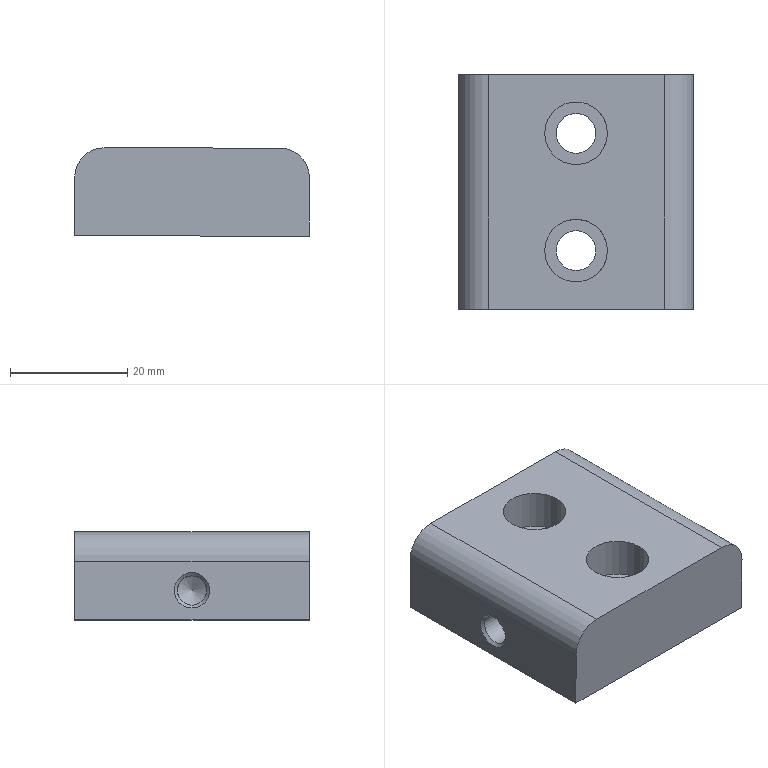Part | STEP file | 冲床-300配套压波_id690_x_t | 1 solid | 18 faces | box 40.015 x 40 x 15.054 mm | volume 21445 mm3 | plane 8 | cylinder 7 | cone 2 | spline 1 | commonest cylinder face diameters 6.8 x2 10 x2 10.7 x2 5 x1
STEP:
#1=CARTESIAN_POINT('',(2190.116,10.,-397.711));
#2=VERTEX_POINT('',#1);
#3=CARTESIAN_POINT('',(2193.516,10.,-397.716));
#4=DIRECTION('',(0.001532,0.,1.));
#5=DIRECTION('',(-1.,0.,0.001532));
#6=AXIS2_PLACEMENT_3D('',#3,#4,#5);
#7=CIRCLE('',#6,3.4);
#8=EDGE_CURVE('',#2,#2,#7,.T.);
#9=ORIENTED_EDGE('',*,*,#8,.F.);
#10=EDGE_LOOP('',(#9));
#11=FACE_BOUND('',#10,.T.);
#12=CARTESIAN_POINT('',(2188.166,10.,-397.708));
#13=VERTEX_POINT('',#12);
#14=CARTESIAN_POINT('',(2193.516,10.,-397.716));
#15=DIRECTION('',(0.001532,0.,1.));
#16=DIRECTION('',(-1.,0.,0.001532));
#17=AXIS2_PLACEMENT_3D('',#14,#15,#16);
#18=CIRCLE('',#17,5.35);
#19=EDGE_CURVE('',#13,#13,#18,.T.);
#20=ORIENTED_EDGE('',*,*,#19,.T.);
#21=EDGE_LOOP('',(#20));
#22=FACE_BOUND('',#21,.T.);
#23=CARTESIAN_POINT('',(2193.516,10.,-397.716));
#24=DIRECTION('',(-0.001532,0.,-1.));
#25=DIRECTION('',(-1.,0.,0.001532));
#26=AXIS2_PLACEMENT_3D('',#23,#24,#25);
#27=PLANE('',#26);
#28=ADVANCED_FACE('',(#11,#22),#27,.F.);
#29=CARTESIAN_POINT('',(2190.103,10.,-405.911));
#30=VERTEX_POINT('',#29);
#31=CARTESIAN_POINT('',(2193.503,10.,-405.916));
#32=DIRECTION('',(0.001532,0.,1.));
#33=DIRECTION('',(-1.,0.,0.001532));
#34=AXIS2_PLACEMENT_3D('',#31,#32,#33);
#35=CIRCLE('',#34,3.4);
#36=EDGE_CURVE('',#30,#30,#35,.T.);
#37=ORIENTED_EDGE('',*,*,#36,.F.);
#38=EDGE_LOOP('',(#37));
#39=FACE_BOUND('',#38,.T.);
#40=ORIENTED_EDGE('',*,*,#8,.T.);
#41=EDGE_LOOP('',(#40));
#42=FACE_BOUND('',#41,.T.);
#43=CARTESIAN_POINT('',(2193.449,10.,-440.916));
#44=DIRECTION('',(-0.001532,0.,-1.));
#45=DIRECTION('',(-1.,0.,0.001532));
#46=AXIS2_PLACEMENT_3D('',#43,#44,#45);
#47=CYLINDRICAL_SURFACE('',#46,3.4);
#48=ADVANCED_FACE('',(#39,#42),#47,.F.);
#49=ORIENTED_EDGE('',*,*,#19,.F.);
#50=EDGE_LOOP('',(#49));
#51=FACE_BOUND('',#50,.T.);
#52=CARTESIAN_POINT('',(2188.176,10.,-390.908));
#53=VERTEX_POINT('',#52);
#54=CARTESIAN_POINT('',(2193.526,10.,-390.916));
#55=DIRECTION('',(-0.001532,0.,-1.));
#56=DIRECTION('',(-1.,0.,0.001532));
#57=AXIS2_PLACEMENT_3D('',#54,#55,#56);
#58=CIRCLE('',#57,5.35);
#59=EDGE_CURVE('',#53,#53,#58,.T.);
#60=ORIENTED_EDGE('',*,*,#59,.F.);
#61=EDGE_LOOP('',(#60));
#62=FACE_BOUND('',#61,.T.);
#63=CARTESIAN_POINT('',(2193.526,10.,-390.916));
#64=DIRECTION('',(-0.001532,0.,-1.));
#65=DIRECTION('',(-1.,0.,0.001532));
#66=AXIS2_PLACEMENT_3D('',#63,#64,#65);
#67=CYLINDRICAL_SURFACE('',#66,5.35);
#68=ADVANCED_FACE('',(#51,#62),#67,.F.);
#69=CARTESIAN_POINT('',(2190.116,-10.,-397.711));
#70=VERTEX_POINT('',#69);
#71=CARTESIAN_POINT('',(2193.516,-10.,-397.716));
#72=DIRECTION('',(0.001532,0.,1.));
#73=DIRECTION('',(-1.,0.,0.001532));
#74=AXIS2_PLACEMENT_3D('',#71,#72,#73);
#75=CIRCLE('',#74,3.4);
#76=EDGE_CURVE('',#70,#70,#75,.T.);
#77=ORIENTED_EDGE('',*,*,#76,.F.);
#78=EDGE_LOOP('',(#77));
#79=FACE_BOUND('',#78,.T.);
#80=CARTESIAN_POINT('',(2188.166,-10.,-397.708));
#81=VERTEX_POINT('',#80);
#82=CARTESIAN_POINT('',(2193.516,-10.,-397.716));
#83=DIRECTION('',(0.001532,0.,1.));
#84=DIRECTION('',(-1.,0.,0.001532));
#85=AXIS2_PLACEMENT_3D('',#82,#83,#84);
#86=CIRCLE('',#85,5.35);
#87=EDGE_CURVE('',#81,#81,#86,.T.);
#88=ORIENTED_EDGE('',*,*,#87,.T.);
#89=EDGE_LOOP('',(#88));
#90=FACE_BOUND('',#89,.T.);
#91=CARTESIAN_POINT('',(2193.516,10.,-397.716));
#92=DIRECTION('',(-0.001532,0.,-1.));
#93=DIRECTION('',(-1.,0.,0.001532));
#94=AXIS2_PLACEMENT_3D('',#91,#92,#93);
#95=PLANE('',#94);
#96=ADVANCED_FACE('',(#79,#90),#95,.F.);
#97=CARTESIAN_POINT('',(2208.526,20.,-390.939));
#98=VERTEX_POINT('',#97);
#99=CARTESIAN_POINT('',(2178.526,20.,-390.893));
#100=VERTEX_POINT('',#99);
#101=CARTESIAN_POINT('',(2203.526,20.,-390.931));
#102=DIRECTION('',(-1.,0.,0.001532));
#103=VECTOR('',#102,1.);
#104=LINE('',#101,#103);
#105=EDGE_CURVE('',#98,#100,#104,.T.);
#106=ORIENTED_EDGE('',*,*,#105,.F.);
#107=CARTESIAN_POINT('',(2213.518,20.,-395.947));
#108=VERTEX_POINT('',#107);
#109=CARTESIAN_POINT('',(2208.518,20.,-395.939));
#110=DIRECTION('',(0.,1.,0.));
#111=DIRECTION('',(0.3358,0.,-0.9419));
#112=AXIS2_PLACEMENT_3D('',#109,#110,#111);
#113=CIRCLE('',#112,5.);
#114=EDGE_CURVE('',#98,#108,#113,.T.);
#115=ORIENTED_EDGE('',*,*,#114,.T.);
#116=CARTESIAN_POINT('',(2213.503,20.,-405.947));
#117=VERTEX_POINT('',#116);
#118=CARTESIAN_POINT('',(2213.503,20.,-405.947));
#119=DIRECTION('',(-0.001532,0.,-1.));
#120=VECTOR('',#119,1.);
#121=LINE('',#118,#120);
#122=EDGE_CURVE('',#108,#117,#121,.T.);
#123=ORIENTED_EDGE('',*,*,#122,.T.);
#124=CARTESIAN_POINT('',(2173.503,20.,-405.885));
#125=VERTEX_POINT('',#124);
#126=CARTESIAN_POINT('',(2203.503,20.,-405.931));
#127=DIRECTION('',(-1.,0.,0.001532));
#128=VECTOR('',#127,1.);
#129=LINE('',#126,#128);
#130=EDGE_CURVE('',#117,#125,#129,.T.);
#131=ORIENTED_EDGE('',*,*,#130,.T.);
#132=CARTESIAN_POINT('',(2173.518,20.,-395.885));
#133=VERTEX_POINT('',#132);
#134=CARTESIAN_POINT('',(2173.503,20.,-405.885));
#135=DIRECTION('',(0.001532,0.,1.));
#136=VECTOR('',#135,1.);
#137=LINE('',#134,#136);
#138=EDGE_CURVE('',#125,#133,#137,.T.);
#139=ORIENTED_EDGE('',*,*,#138,.T.);
#140=CARTESIAN_POINT('',(2178.518,20.,-395.893));
#141=DIRECTION('',(0.,1.,0.));
#142=DIRECTION('',(0.3358,0.,-0.9419));
#143=AXIS2_PLACEMENT_3D('',#140,#141,#142);
#144=CIRCLE('',#143,5.);
#145=EDGE_CURVE('',#133,#100,#144,.T.);
#146=ORIENTED_EDGE('',*,*,#145,.T.);
#147=EDGE_LOOP('',(#106,#115,#123,#131,#139,#146));
#148=FACE_OUTER_BOUND('',#147,.T.);
#149=CARTESIAN_POINT('',(2203.503,20.,-405.931));
#150=DIRECTION('',(0.,-1.,0.));
#151=DIRECTION('',(1.,0.,-0.001532));
#152=AXIS2_PLACEMENT_3D('',#149,#150,#151);
#153=PLANE('',#152);
#154=ADVANCED_FACE('',(#148),#153,.F.);
#155=CARTESIAN_POINT('',(2173.518,-20.,-395.885));
#156=VERTEX_POINT('',#155);
#157=CARTESIAN_POINT('',(2173.518,15.,-395.885));
#158=DIRECTION('',(0.,1.,0.));
#159=VECTOR('',#158,1.);
#160=LINE('',#157,#159);
#161=EDGE_CURVE('',#156,#133,#160,.T.);
#162=ORIENTED_EDGE('',*,*,#161,.T.);
#163=ORIENTED_EDGE('',*,*,#138,.F.);
#164=CARTESIAN_POINT('',(2173.503,-20.,-405.885));
#165=VERTEX_POINT('',#164);
#166=CARTESIAN_POINT('',(2173.503,15.,-405.885));
#167=DIRECTION('',(0.,-1.,0.));
#168=VECTOR('',#167,1.);
#169=LINE('',#166,#168);
#170=EDGE_CURVE('',#125,#165,#169,.T.);
#171=ORIENTED_EDGE('',*,*,#170,.T.);
#172=CARTESIAN_POINT('',(2173.503,-20.,-405.885));
#173=DIRECTION('',(0.001532,0.,1.));
#174=VECTOR('',#173,1.);
#175=LINE('',#172,#174);
#176=EDGE_CURVE('',#165,#156,#175,.T.);
#177=ORIENTED_EDGE('',*,*,#176,.T.);
#178=EDGE_LOOP('',(#162,#163,#171,#177));
#179=FACE_BOUND('',#178,.T.);
#180=CARTESIAN_POINT('',(2173.517,-1.657,-398.382));
#181=VERTEX_POINT('',#180);
#182=CARTESIAN_POINT('',(2173.517,1.658,-398.383));
#183=VERTEX_POINT('',#182);
#184=CARTESIAN_POINT('',(2173.511,0.,-400.885));
#185=DIRECTION('',(1.,0.,-0.001532));
#186=DIRECTION('',(-0.001532,0.,-1.));
#187=AXIS2_PLACEMENT_3D('',#184,#185,#186);
#188=CIRCLE('',#187,3.004);
#189=EDGE_CURVE('',#181,#183,#188,.T.);
#190=ORIENTED_EDGE('',*,*,#189,.T.);
#191=CARTESIAN_POINT('',(2173.515,1.66,-398.381));
#192=CARTESIAN_POINT('',(2173.515,1.427,-398.195));
#193=CARTESIAN_POINT('',(2173.515,1.158,-398.046));
#194=CARTESIAN_POINT('',(2173.515,0.8765,-397.947));
#195=CARTESIAN_POINT('',(2173.515,0.7375,-397.898));
#196=CARTESIAN_POINT('',(2173.515,0.594,-397.861));
#197=CARTESIAN_POINT('',(2173.515,0.4488,-397.836));
#198=CARTESIAN_POINT('',(2173.516,0.1563,-397.786));
#199=CARTESIAN_POINT('',(2173.516,-0.1488,-397.786));
#200=CARTESIAN_POINT('',(2173.515,-0.4414,-397.835));
#201=CARTESIAN_POINT('',(2173.515,-0.7342,-397.885));
#202=CARTESIAN_POINT('',(2173.515,-1.022,-397.985));
#203=CARTESIAN_POINT('',(2173.515,-1.282,-398.129));
#204=CARTESIAN_POINT('',(2173.515,-1.414,-398.202));
#205=CARTESIAN_POINT('',(2173.515,-1.541,-398.286));
#206=CARTESIAN_POINT('',(2173.515,-1.659,-398.381));
#207=B_SPLINE_CURVE_WITH_KNOTS('',3,(#191,#192,#193,#194,#195,#196,#197,#198,#199,#200,#201,#202,#203,#204,#205,#206),.UNSPECIFIED.,.F.,.F.,(4,3,3,3,3,4),(0.,0.2513,0.3739,0.6237,0.8736,1.),.UNSPECIFIED.);
#208=EDGE_CURVE('',#183,#181,#207,.T.);
#209=ORIENTED_EDGE('',*,*,#208,.T.);
#210=EDGE_LOOP('',(#190,#209));
#211=FACE_BOUND('',#210,.T.);
#212=CARTESIAN_POINT('',(2173.503,15.,-405.885));
#213=DIRECTION('',(1.,0.,-0.001532));
#214=DIRECTION('',(0.,-1.,0.));
#215=AXIS2_PLACEMENT_3D('',#212,#213,#214);
#216=PLANE('',#215);
#217=ADVANCED_FACE('',(#179,#211),#216,.F.);
#218=CARTESIAN_POINT('',(2213.518,-20.,-395.947));
#219=VERTEX_POINT('',#218);
#220=CARTESIAN_POINT('',(2213.503,-20.,-405.947));
#221=VERTEX_POINT('',#220);
#222=CARTESIAN_POINT('',(2213.503,-20.,-405.947));
#223=DIRECTION('',(-0.001532,0.,-1.));
#224=VECTOR('',#223,1.);
#225=LINE('',#222,#224);
#226=EDGE_CURVE('',#219,#221,#225,.T.);
#227=ORIENTED_EDGE('',*,*,#226,.F.);
#228=CARTESIAN_POINT('',(2208.526,-20.,-390.939));
#229=VERTEX_POINT('',#228);
#230=CARTESIAN_POINT('',(2208.518,-20.,-395.939));
#231=DIRECTION('',(0.,-1.,0.));
#232=DIRECTION('',(0.3358,0.,-0.9419));
#233=AXIS2_PLACEMENT_3D('',#230,#231,#232);
#234=CIRCLE('',#233,5.);
#235=EDGE_CURVE('',#219,#229,#234,.T.);
#236=ORIENTED_EDGE('',*,*,#235,.T.);
#237=CARTESIAN_POINT('',(2178.526,-20.,-390.893));
#238=VERTEX_POINT('',#237);
#239=CARTESIAN_POINT('',(2203.526,-20.,-390.931));
#240=DIRECTION('',(-1.,0.,0.001532));
#241=VECTOR('',#240,1.);
#242=LINE('',#239,#241);
#243=EDGE_CURVE('',#229,#238,#242,.T.);
#244=ORIENTED_EDGE('',*,*,#243,.T.);
#245=CARTESIAN_POINT('',(2178.518,-20.,-395.893));
#246=DIRECTION('',(0.,-1.,0.));
#247=DIRECTION('',(0.3358,0.,-0.9419));
#248=AXIS2_PLACEMENT_3D('',#245,#246,#247);
#249=CIRCLE('',#248,5.);
#250=EDGE_CURVE('',#238,#156,#249,.T.);
#251=ORIENTED_EDGE('',*,*,#250,.T.);
#252=ORIENTED_EDGE('',*,*,#176,.F.);
#253=CARTESIAN_POINT('',(2203.503,-20.,-405.931));
#254=DIRECTION('',(-1.,0.,0.001532));
#255=VECTOR('',#254,1.);
#256=LINE('',#253,#255);
#257=EDGE_CURVE('',#221,#165,#256,.T.);
#258=ORIENTED_EDGE('',*,*,#257,.F.);
#259=EDGE_LOOP('',(#227,#236,#244,#251,#252,#258));
#260=FACE_OUTER_BOUND('',#259,.T.);
#261=CARTESIAN_POINT('',(2203.503,-20.,-405.931));
#262=DIRECTION('',(0.,-1.,0.));
#263=DIRECTION('',(1.,0.,-0.001532));
#264=AXIS2_PLACEMENT_3D('',#261,#262,#263);
#265=PLANE('',#264);
#266=ADVANCED_FACE('',(#260),#265,.T.);
#267=ORIENTED_EDGE('',*,*,#122,.F.);
#268=CARTESIAN_POINT('',(2213.518,15.,-395.947));
#269=DIRECTION('',(0.,-1.,0.));
#270=VECTOR('',#269,1.);
#271=LINE('',#268,#270);
#272=EDGE_CURVE('',#108,#219,#271,.T.);
#273=ORIENTED_EDGE('',*,*,#272,.T.);
#274=ORIENTED_EDGE('',*,*,#226,.T.);
#275=CARTESIAN_POINT('',(2213.503,15.,-405.947));
#276=DIRECTION('',(0.,1.,0.));
#277=VECTOR('',#276,1.);
#278=LINE('',#275,#277);
#279=EDGE_CURVE('',#221,#117,#278,.T.);
#280=ORIENTED_EDGE('',*,*,#279,.T.);
#281=EDGE_LOOP('',(#267,#273,#274,#280));
#282=FACE_OUTER_BOUND('',#281,.T.);
#283=CARTESIAN_POINT('',(2213.503,15.,-405.947));
#284=DIRECTION('',(-1.,0.,0.001532));
#285=DIRECTION('',(0.,-1.,0.));
#286=AXIS2_PLACEMENT_3D('',#283,#284,#285);
#287=PLANE('',#286);
#288=ADVANCED_FACE('',(#282),#287,.F.);
#289=CARTESIAN_POINT('',(2190.103,-10.,-405.911));
#290=VERTEX_POINT('',#289);
#291=CARTESIAN_POINT('',(2193.503,-10.,-405.916));
#292=DIRECTION('',(-0.001532,0.,-1.));
#293=DIRECTION('',(-1.,0.,0.001532));
#294=AXIS2_PLACEMENT_3D('',#291,#292,#293);
#295=CIRCLE('',#294,3.4);
#296=EDGE_CURVE('',#290,#290,#295,.T.);
#297=ORIENTED_EDGE('',*,*,#296,.T.);
#298=EDGE_LOOP('',(#297));
#299=FACE_BOUND('',#298,.T.);
#300=ORIENTED_EDGE('',*,*,#76,.T.);
#301=EDGE_LOOP('',(#300));
#302=FACE_BOUND('',#301,.T.);
#303=CARTESIAN_POINT('',(2193.449,-10.,-440.916));
#304=DIRECTION('',(-0.001532,0.,-1.));
#305=DIRECTION('',(-1.,0.,0.001532));
#306=AXIS2_PLACEMENT_3D('',#303,#304,#305);
#307=CYLINDRICAL_SURFACE('',#306,3.4);
#308=ADVANCED_FACE('',(#299,#302),#307,.F.);
#309=ORIENTED_EDGE('',*,*,#36,.T.);
#310=EDGE_LOOP('',(#309));
#311=FACE_BOUND('',#310,.T.);
#312=ORIENTED_EDGE('',*,*,#296,.F.);
#313=EDGE_LOOP('',(#312));
#314=FACE_BOUND('',#313,.T.);
#315=ORIENTED_EDGE('',*,*,#279,.F.);
#316=ORIENTED_EDGE('',*,*,#257,.T.);
#317=ORIENTED_EDGE('',*,*,#170,.F.);
#318=ORIENTED_EDGE('',*,*,#130,.F.);
#319=EDGE_LOOP('',(#315,#316,#317,#318));
#320=FACE_BOUND('',#319,.T.);
#321=CARTESIAN_POINT('',(2203.503,15.,-405.931));
#322=DIRECTION('',(-0.001532,0.,-1.));
#323=DIRECTION('',(1.,0.,-0.001532));
#324=AXIS2_PLACEMENT_3D('',#321,#322,#323);
#325=PLANE('',#324);
#326=ADVANCED_FACE('',(#311,#314,#320),#325,.T.);
#327=ORIENTED_EDGE('',*,*,#87,.F.);
#328=EDGE_LOOP('',(#327));
#329=FACE_BOUND('',#328,.T.);
#330=CARTESIAN_POINT('',(2188.176,-10.,-390.908));
#331=VERTEX_POINT('',#330);
#332=CARTESIAN_POINT('',(2193.526,-10.,-390.916));
#333=DIRECTION('',(-0.001532,0.,-1.));
#334=DIRECTION('',(-1.,0.,0.001532));
#335=AXIS2_PLACEMENT_3D('',#332,#333,#334);
#336=CIRCLE('',#335,5.35);
#337=EDGE_CURVE('',#331,#331,#336,.T.);
#338=ORIENTED_EDGE('',*,*,#337,.F.);
#339=EDGE_LOOP('',(#338));
#340=FACE_BOUND('',#339,.T.);
#341=CARTESIAN_POINT('',(2193.526,-10.,-390.916));
#342=DIRECTION('',(-0.001532,0.,-1.));
#343=DIRECTION('',(-1.,0.,0.001532));
#344=AXIS2_PLACEMENT_3D('',#341,#342,#343);
#345=CYLINDRICAL_SURFACE('',#344,5.35);
#346=ADVANCED_FACE('',(#329,#340),#345,.F.);
#347=ORIENTED_EDGE('',*,*,#59,.T.);
#348=EDGE_LOOP('',(#347));
#349=FACE_BOUND('',#348,.T.);
#350=ORIENTED_EDGE('',*,*,#337,.T.);
#351=EDGE_LOOP('',(#350));
#352=FACE_BOUND('',#351,.T.);
#353=ORIENTED_EDGE('',*,*,#243,.F.);
#354=CARTESIAN_POINT('',(2208.526,15.,-390.939));
#355=DIRECTION('',(0.,1.,0.));
#356=VECTOR('',#355,1.);
#357=LINE('',#354,#356);
#358=EDGE_CURVE('',#229,#98,#357,.T.);
#359=ORIENTED_EDGE('',*,*,#358,.T.);
#360=ORIENTED_EDGE('',*,*,#105,.T.);
#361=CARTESIAN_POINT('',(2178.526,15.,-390.893));
#362=DIRECTION('',(0.,-1.,0.));
#363=VECTOR('',#362,1.);
#364=LINE('',#361,#363);
#365=EDGE_CURVE('',#100,#238,#364,.T.);
#366=ORIENTED_EDGE('',*,*,#365,.T.);
#367=EDGE_LOOP('',(#353,#359,#360,#366));
#368=FACE_BOUND('',#367,.T.);
#369=CARTESIAN_POINT('',(2203.526,15.,-390.931));
#370=DIRECTION('',(-0.001532,0.,-1.));
#371=DIRECTION('',(1.,0.,-0.001532));
#372=AXIS2_PLACEMENT_3D('',#369,#370,#371);
#373=PLANE('',#372);
#374=ADVANCED_FACE('',(#349,#352,#368),#373,.F.);
#375=ORIENTED_EDGE('',*,*,#235,.F.);
#376=ORIENTED_EDGE('',*,*,#272,.F.);
#377=ORIENTED_EDGE('',*,*,#114,.F.);
#378=ORIENTED_EDGE('',*,*,#358,.F.);
#379=EDGE_LOOP('',(#375,#376,#377,#378));
#380=FACE_OUTER_BOUND('',#379,.T.);
#381=CARTESIAN_POINT('',(2208.518,15.,-395.939));
#382=DIRECTION('',(0.,1.,0.));
#383=DIRECTION('',(-0.3358,0.,0.9419));
#384=AXIS2_PLACEMENT_3D('',#381,#382,#383);
#385=CYLINDRICAL_SURFACE('',#384,5.);
#386=ADVANCED_FACE('',(#380),#385,.T.);
#387=ORIENTED_EDGE('',*,*,#145,.F.);
#388=ORIENTED_EDGE('',*,*,#161,.F.);
#389=ORIENTED_EDGE('',*,*,#250,.F.);
#390=ORIENTED_EDGE('',*,*,#365,.F.);
#391=EDGE_LOOP('',(#387,#388,#389,#390));
#392=FACE_OUTER_BOUND('',#391,.T.);
#393=CARTESIAN_POINT('',(2178.518,15.,-395.893));
#394=DIRECTION('',(0.,-1.,0.));
#395=DIRECTION('',(0.3358,0.,-0.9419));
#396=AXIS2_PLACEMENT_3D('',#393,#394,#395);
#397=CYLINDRICAL_SURFACE('',#396,5.);
#398=ADVANCED_FACE('',(#392),#397,.T.);
#399=CARTESIAN_POINT('',(2188.511,0.,-403.408));
#400=VERTEX_POINT('',#399);
#401=CARTESIAN_POINT('',(2188.515,0.,-400.908));
#402=DIRECTION('',(-1.,0.,0.001532));
#403=DIRECTION('',(-0.001532,0.,-1.));
#404=AXIS2_PLACEMENT_3D('',#401,#402,#403);
#405=CIRCLE('',#404,2.5);
#406=EDGE_CURVE('',#400,#400,#405,.T.);
#407=ORIENTED_EDGE('',*,*,#406,.T.);
#408=EDGE_LOOP('',(#407));
#409=FACE_BOUND('',#408,.T.);
#410=CARTESIAN_POINT('',(2190.017,0.,-400.911));
#411=VERTEX_POINT('',#410);
#412=VERTEX_LOOP('',#411);
#413=FACE_BOUND('',#412,.T.);
#414=CARTESIAN_POINT('',(2188.515,0.,-400.908));
#415=DIRECTION('',(-1.,0.,0.001532));
#416=DIRECTION('',(0.001532,0.,1.));
#417=AXIS2_PLACEMENT_3D('',#414,#415,#416);
#418=CONICAL_SURFACE('',#417,2.5,59.);
#419=ADVANCED_FACE('',(#409,#413),#418,.F.);
#420=CARTESIAN_POINT('',(2174.018,1.382,-398.803));
#421=VERTEX_POINT('',#420);
#422=CARTESIAN_POINT('',(2174.018,-1.382,-398.803));
#423=VERTEX_POINT('',#422);
#424=CARTESIAN_POINT('',(2174.015,0.,-400.886));
#425=DIRECTION('',(-1.,0.,0.001532));
#426=DIRECTION('',(-0.001532,0.,-1.));
#427=AXIS2_PLACEMENT_3D('',#424,#425,#426);
#428=CIRCLE('',#427,2.5);
#429=EDGE_CURVE('',#421,#423,#428,.T.);
#430=ORIENTED_EDGE('',*,*,#429,.T.);
#431=CARTESIAN_POINT('',(2174.018,-1.382,-398.803));
#432=CARTESIAN_POINT('',(2174.05,-0.567,-398.262));
#433=CARTESIAN_POINT('',(2174.05,0.5699,-398.264));
#434=CARTESIAN_POINT('',(2174.018,1.382,-398.803));
#435=B_SPLINE_CURVE_WITH_KNOTS('',3,(#431,#432,#433,#434),.UNSPECIFIED.,.F.,.F.,(4,4),(0.,1.),.UNSPECIFIED.);
#436=EDGE_CURVE('',#423,#421,#435,.T.);
#437=ORIENTED_EDGE('',*,*,#436,.T.);
#438=EDGE_LOOP('',(#430,#437));
#439=FACE_BOUND('',#438,.T.);
#440=ORIENTED_EDGE('',*,*,#406,.F.);
#441=EDGE_LOOP('',(#440));
#442=FACE_BOUND('',#441,.T.);
#443=CARTESIAN_POINT('',(2173.515,0.,-400.885));
#444=DIRECTION('',(1.,0.,-0.001532));
#445=DIRECTION('',(-0.001532,0.,-1.));
#446=AXIS2_PLACEMENT_3D('',#443,#444,#445);
#447=CYLINDRICAL_SURFACE('',#446,2.5);
#448=ADVANCED_FACE('',(#439,#442),#447,.F.);
#449=CARTESIAN_POINT('',(2174.018,1.382,-398.803));
#450=CARTESIAN_POINT('',(2173.851,1.474,-398.664));
#451=CARTESIAN_POINT('',(2173.685,1.566,-398.525));
#452=CARTESIAN_POINT('',(2173.518,1.658,-398.385));
#453=B_SPLINE_CURVE_WITH_KNOTS('',3,(#449,#450,#451,#452),.UNSPECIFIED.,.F.,.F.,(4,4),(0.,1.),.UNSPECIFIED.);
#454=EDGE_CURVE('',#421,#183,#453,.T.);
#455=ORIENTED_EDGE('',*,*,#454,.F.);
#456=ORIENTED_EDGE('',*,*,#436,.F.);
#457=CARTESIAN_POINT('',(2173.518,-1.658,-398.385));
#458=CARTESIAN_POINT('',(2173.685,-1.566,-398.525));
#459=CARTESIAN_POINT('',(2173.851,-1.474,-398.664));
#460=CARTESIAN_POINT('',(2174.018,-1.382,-398.803));
#461=B_SPLINE_CURVE_WITH_KNOTS('',3,(#457,#458,#459,#460),.UNSPECIFIED.,.F.,.F.,(4,4),(0.,1.),.UNSPECIFIED.);
#462=EDGE_CURVE('',#181,#423,#461,.T.);
#463=ORIENTED_EDGE('',*,*,#462,.F.);
#464=ORIENTED_EDGE('',*,*,#208,.F.);
#465=EDGE_LOOP('',(#455,#456,#463,#464));
#466=FACE_OUTER_BOUND('',#465,.T.);
#467=CARTESIAN_POINT('',(2173.482,1.679,-398.355));
#468=CARTESIAN_POINT('',(2173.518,0.6859,-397.601));
#469=CARTESIAN_POINT('',(2173.518,-0.8005,-397.606));
#470=CARTESIAN_POINT('',(2173.462,-2.158,-398.753));
#471=CARTESIAN_POINT('',(2173.446,-2.56,-399.092));
#472=CARTESIAN_POINT('',(2173.432,-2.886,-399.368));
#473=CARTESIAN_POINT('',(2174.018,1.382,-398.803));
#474=CARTESIAN_POINT('',(2174.05,0.5647,-398.248));
#475=CARTESIAN_POINT('',(2174.05,-0.659,-398.251));
#476=CARTESIAN_POINT('',(2174.001,-1.777,-399.096));
#477=CARTESIAN_POINT('',(2173.986,-2.107,-399.346));
#478=CARTESIAN_POINT('',(2173.974,-2.376,-399.549));
#479=B_SPLINE_SURFACE_WITH_KNOTS('',1,3,((#467,#468,#469,#470,#471,#472),(#473,#474,#475,#476,#477,#478)),.UNSPECIFIED.,.F.,.F.,.F.,(2,2),(4,1,1,4),(0.,1.),(0.,0.7042,0.7599,1.),.UNSPECIFIED.);
#480=ADVANCED_FACE('',(#466),#479,.T.);
#481=ORIENTED_EDGE('',*,*,#462,.T.);
#482=ORIENTED_EDGE('',*,*,#429,.F.);
#483=ORIENTED_EDGE('',*,*,#454,.T.);
#484=ORIENTED_EDGE('',*,*,#189,.F.);
#485=EDGE_LOOP('',(#481,#482,#483,#484));
#486=FACE_OUTER_BOUND('',#485,.T.);
#487=CARTESIAN_POINT('',(2173.515,0.,-400.885));
#488=DIRECTION('',(-1.,0.,0.001532));
#489=DIRECTION('',(0.001532,0.,1.));
#490=AXIS2_PLACEMENT_3D('',#487,#488,#489);
#491=CONICAL_SURFACE('',#490,3.,45.);
#492=ADVANCED_FACE('',(#486),#491,.F.);
#493=CLOSED_SHELL('',(#28,#48,#68,#96,#154,#217,#266,#288,#308,#326,#346,#374,#386,#398,#419,#448,#480,#492));
#494=MANIFOLD_SOLID_BREP('',#493);
#495=(LENGTH_UNIT()NAMED_UNIT(*)SI_UNIT(.MILLI.,.METRE.));
#496=UNCERTAINTY_MEASURE_WITH_UNIT(LENGTH_MEASURE(0.0508),#495,'','');
#497=(NAMED_UNIT(*)PLANE_ANGLE_UNIT()SI_UNIT($,.RADIAN.));
#498=PLANE_ANGLE_MEASURE_WITH_UNIT(PLANE_ANGLE_MEASURE(0.01745),#497);
#499=DIMENSIONAL_EXPONENTS(0.,0.,0.,0.,0.,0.,0.);
#500=(CONVERSION_BASED_UNIT('DEGREE',#498)NAMED_UNIT(#499)PLANE_ANGLE_UNIT());
#501=(NAMED_UNIT(*)SI_UNIT($,.STERADIAN.)SOLID_ANGLE_UNIT());
#502=(GEOMETRIC_REPRESENTATION_CONTEXT(3)GLOBAL_UNCERTAINTY_ASSIGNED_CONTEXT((#496))GLOBAL_UNIT_ASSIGNED_CONTEXT((#495,#500,#501))REPRESENTATION_CONTEXT('',''));
#503=ADVANCED_BREP_SHAPE_REPRESENTATION('',(#494),#502);